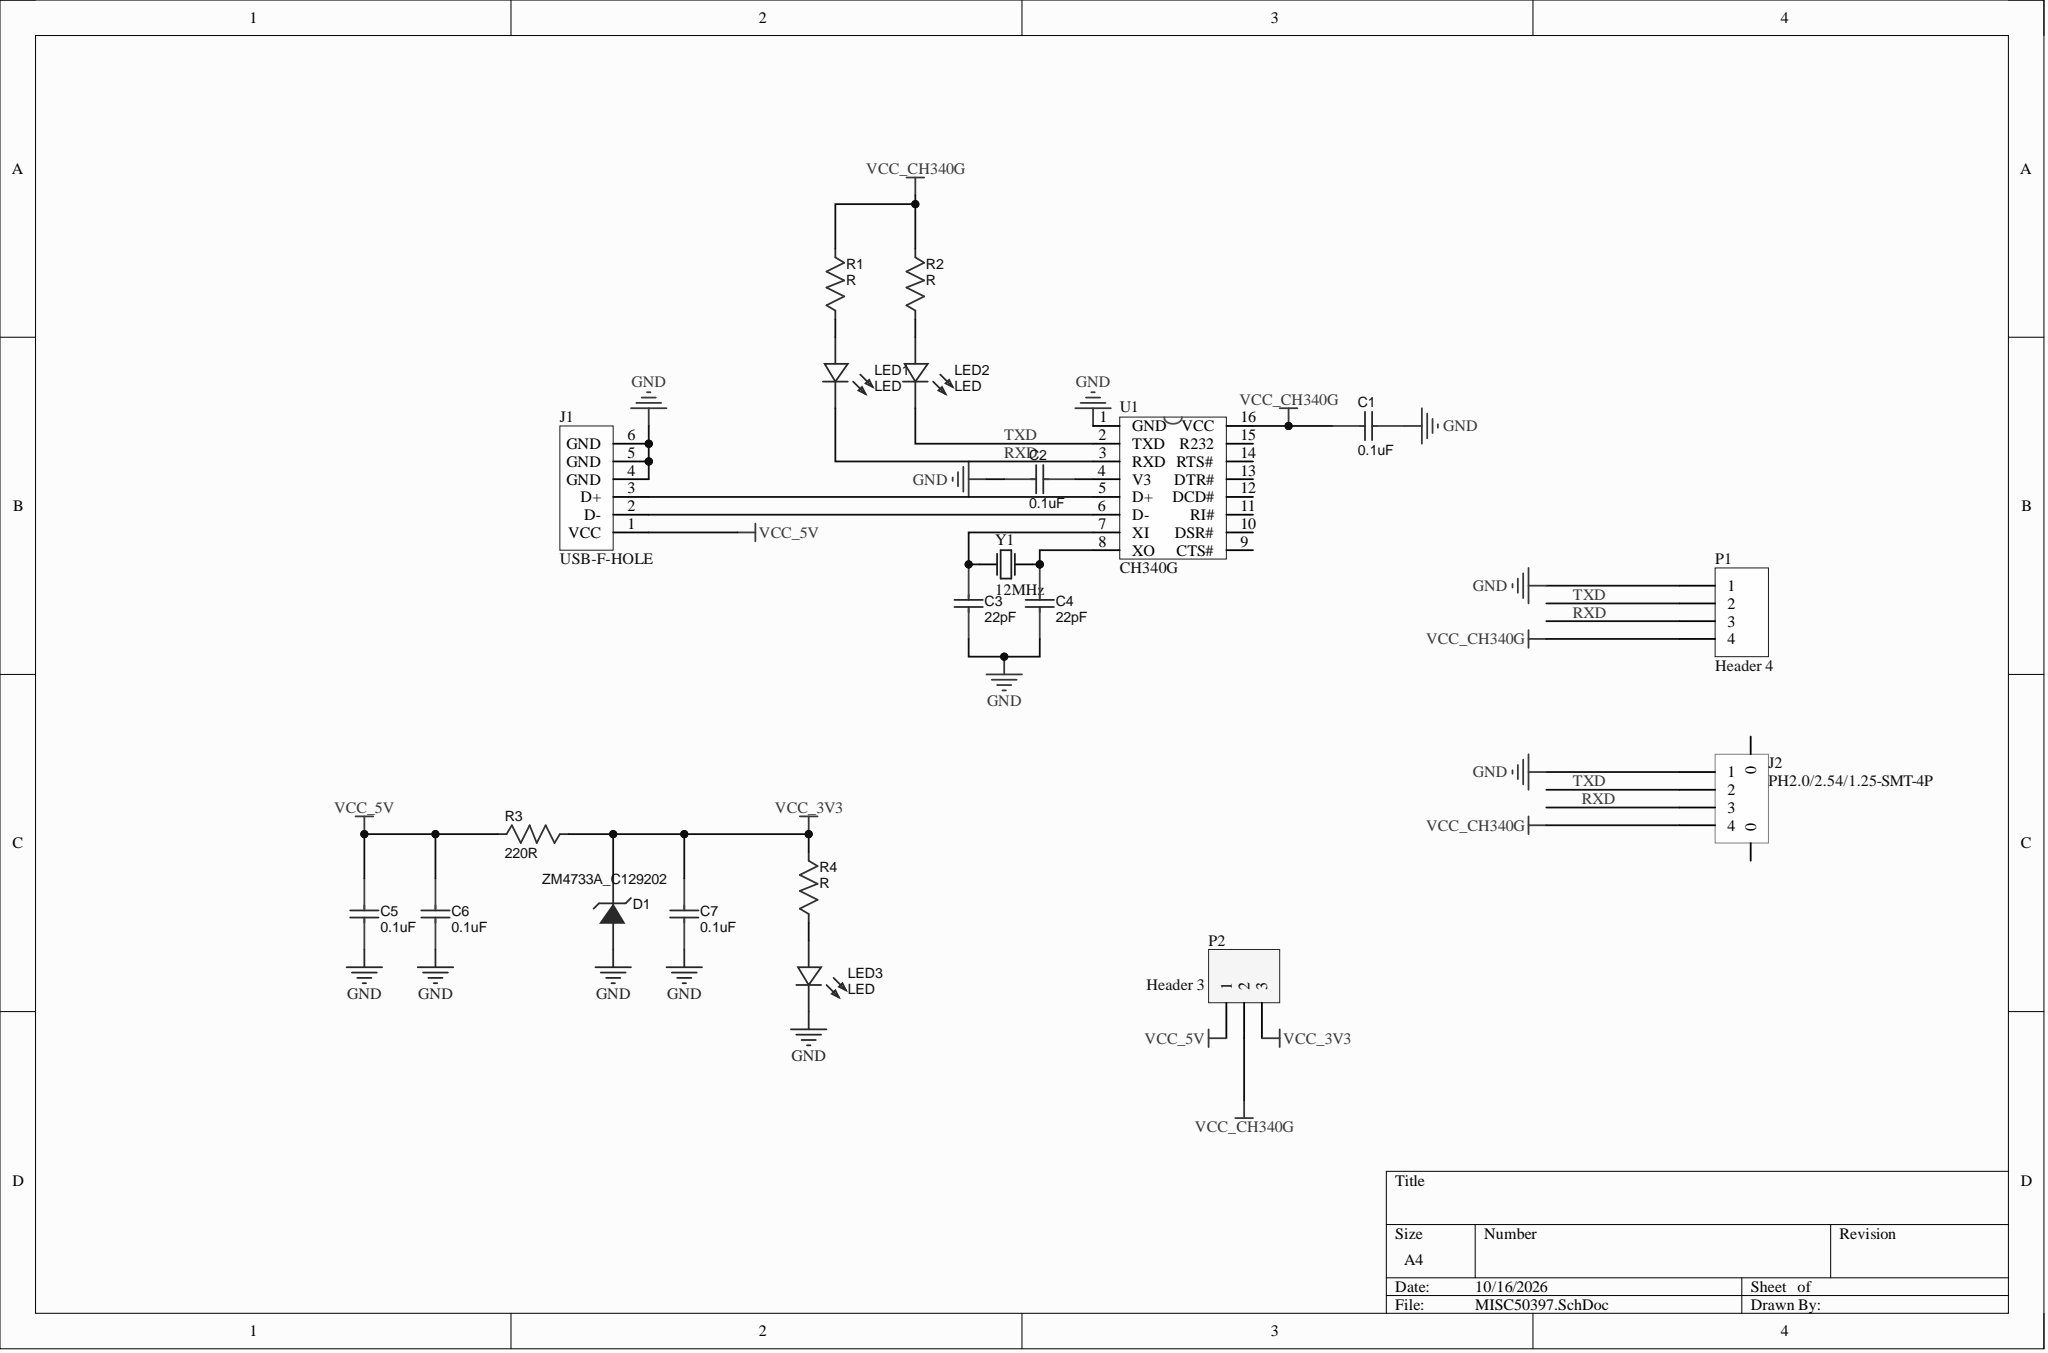Circuit board | Altium Designer | 21 parts | 14 nets
Bill of materials:
Comment,Description,Designator,Footprint,LibRef,Quantity
"0.1uF","","C1, C2, C5, C6, C7","CAP0603","C","5"
"22pF","","C3, C4","CAP0603","C","2"
"ZM4733A_C129202","","D1","LL-41","ZM4733A_C129202","1"
"USB-F-HOLE","","J1","USB-F-HOLE","USB-F-HOLE","1"
"PH2.0/2.54/1.25-SMT-4P","","J2","PH2.0-4P-WT","PH2.0/2.54/1.25-SMT-4P","1"
"LED","","LED1, LED2, LED3","LED-0603_RED","LED","3"
"Header 4","Header, 4-Pin","P1","HDR1X4","Header 4","1"
"Header 3","Header, 3-Pin","P2","HDR1X3","Header 3","1"
"R","","R1, R2, R4","RES0603","R","3"
"220R","","R3","RES0603","R","1"
"CH340G","USB2UART","U1","SOP16M","CH340G","1"
"12MHz","","Y1","XTAL-5.08","XTAL","1"
Netlist (Protel format):
[
C1
CAP0603
0.1uF



]
[
C2
CAP0603
0.1uF



]
[
C3
CAP0603
22pF



]
[
C4
CAP0603
22pF



]
[
C5
CAP0603
0.1uF



]
[
C6
CAP0603
0.1uF



]
[
C7
CAP0603
0.1uF



]
[
D1
LL-41
ZM4733A_C129202



]
[
J1
USB-F-HOLE
USB-F-HOLE



]
[
J2
PH2.0-4P-WT
PH2.0/2.54/1.25-SMT-4P



]
[
LED1
LED-0603_RED
LED



]
[
LED2
LED-0603_RED
LED



]
[
LED3
LED-0603_RED
LED



]
[
P1
HDR1X4
Header 4



]
[
P2
HDR1X3
Header 3



]
[
R1
RES0603
R



]
[
R2
RES0603
R



]
[
R3
RES0603
220R



]
[
R4
RES0603
R



]
[
U1
SOP16M
CH340G



]
[
Y1
XTAL-5.08
12MHz



]
(
VCC_CH340G
C1-1
J2-4
P1-4
P2-2
R1-2
R2-2
U1-16
)
(
VCC_5V
C5-2
C6-2
J1-1
P2-1
R3-1
)
(
VCC_3V3
C7-2
D1-2
P2-3
R3-2
R4-2
)
(
TXD
J2-2
LED2-2
P1-2
U1-2
)
(
RXD
J2-3
LED1-2
P1-3
U1-3
)
(
NetLED3_1
LED3-1
R4-1
)
(
NetLED2_1
LED2-1
R2-1
)
(
NetLED1_1
LED1-1
R1-1
)
(
NetJ1_3
J1-3
U1-5
)
(
NetJ1_2
J1-2
U1-6
)
(
NetC4_2
C4-2
U1-8
Y1-1
)
(
NetC3_2
C3-2
U1-7
Y1-2
)
(
NetC2_1
C2-1
U1-4
)
(
GND
C1-2
C2-2
C3-1
C4-1
C5-1
C6-1
C7-1
D1-1
J1-4
J1-5
J1-6
J2-1
LED3-2
P1-1
U1-1
)